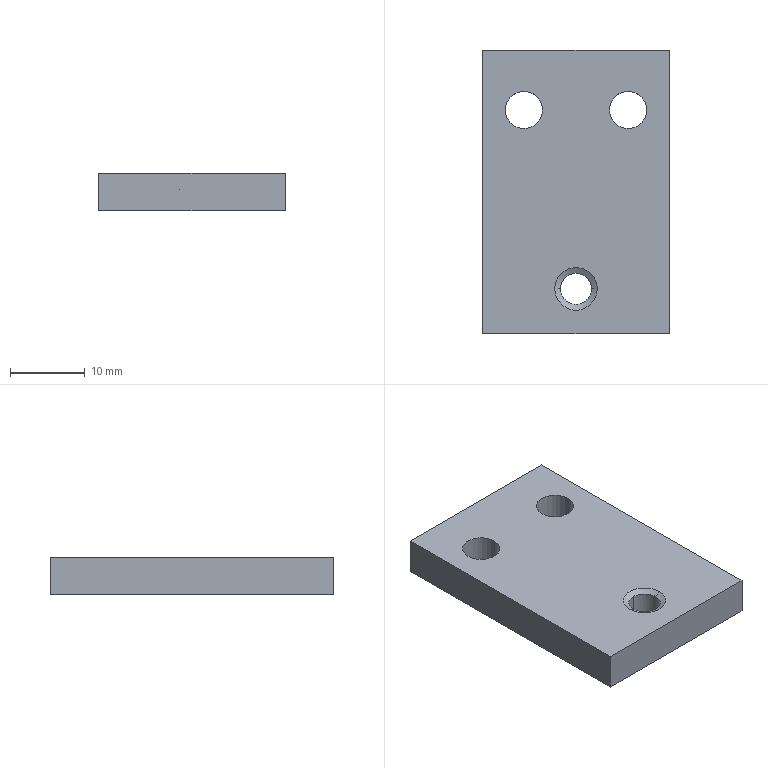Part | NX | 1 solid | 14 faces | box 25 x 38 x 5 mm | volume 4482 mm3 | plane 6 | cylinder 6 | cone 2 | commonest cylinder face diameters 5 x4 4.2 x2
STEP:
#1=CARTESIAN_POINT('',(-12.5,-20.5,-2.5));
#2=VERTEX_POINT('',#1);
#3=CARTESIAN_POINT('',(-12.5,17.5,-2.5));
#4=VERTEX_POINT('',#3);
#5=CARTESIAN_POINT('',(-12.5,0.,-2.5));
#6=DIRECTION('',(0.,1.,0.));
#7=VECTOR('',#6,1000.);
#8=LINE('',#5,#7);
#9=EDGE_CURVE('',#2,#4,#8,.T.);
#10=ORIENTED_EDGE('',*,*,#9,.T.);
#11=CARTESIAN_POINT('',(12.5,17.5,-2.5));
#12=VERTEX_POINT('',#11);
#13=CARTESIAN_POINT('',(0.,17.5,-2.5));
#14=DIRECTION('',(-1.,0.,0.));
#15=VECTOR('',#14,1000.);
#16=LINE('',#13,#15);
#17=EDGE_CURVE('',#12,#4,#16,.T.);
#18=ORIENTED_EDGE('',*,*,#17,.F.);
#19=CARTESIAN_POINT('',(12.5,-20.5,-2.5));
#20=VERTEX_POINT('',#19);
#21=CARTESIAN_POINT('',(12.5,0.,-2.5));
#22=DIRECTION('',(0.,-1.,0.));
#23=VECTOR('',#22,1000.);
#24=LINE('',#21,#23);
#25=EDGE_CURVE('',#12,#20,#24,.T.);
#26=ORIENTED_EDGE('',*,*,#25,.T.);
#27=CARTESIAN_POINT('',(0.,-20.5,-2.5));
#28=DIRECTION('',(1.,0.,0.));
#29=VECTOR('',#28,1000.);
#30=LINE('',#27,#29);
#31=EDGE_CURVE('',#2,#20,#30,.T.);
#32=ORIENTED_EDGE('',*,*,#31,.F.);
#33=EDGE_LOOP('',(#10,#18,#26,#32));
#34=FACE_BOUND('',#33,.T.);
#35=CARTESIAN_POINT('',(-4.5,9.5,-2.5));
#36=VERTEX_POINT('',#35);
#37=CARTESIAN_POINT('',(-9.5,9.5,-2.5));
#38=VERTEX_POINT('',#37);
#39=CARTESIAN_POINT('',(-7.,9.5,-2.5));
#40=DIRECTION('',(0.,0.,-1.));
#41=DIRECTION('',(-1.,0.,0.));
#42=AXIS2_PLACEMENT_3D('',#39,#40,#41);
#43=CIRCLE('',#42,2.5);
#44=EDGE_CURVE('',#36,#38,#43,.T.);
#45=ORIENTED_EDGE('',*,*,#44,.F.);
#46=CARTESIAN_POINT('',(-7.,9.5,-2.5));
#47=DIRECTION('',(0.,0.,-1.));
#48=DIRECTION('',(-1.,0.,0.));
#49=AXIS2_PLACEMENT_3D('',#46,#47,#48);
#50=CIRCLE('',#49,2.5);
#51=EDGE_CURVE('',#38,#36,#50,.T.);
#52=ORIENTED_EDGE('',*,*,#51,.F.);
#53=EDGE_LOOP('',(#45,#52));
#54=FACE_BOUND('',#53,.T.);
#55=CARTESIAN_POINT('',(0.,-12.4,-2.5));
#56=VERTEX_POINT('',#55);
#57=CARTESIAN_POINT('',(0.,-16.6,-2.5));
#58=VERTEX_POINT('',#57);
#59=CARTESIAN_POINT('',(0.,-14.5,-2.5));
#60=DIRECTION('',(0.,0.,1.));
#61=DIRECTION('',(0.,-1.,0.));
#62=AXIS2_PLACEMENT_3D('',#59,#60,#61);
#63=CIRCLE('',#62,2.1);
#64=EDGE_CURVE('',#56,#58,#63,.T.);
#65=ORIENTED_EDGE('',*,*,#64,.T.);
#66=CARTESIAN_POINT('',(0.,-14.5,-2.5));
#67=DIRECTION('',(0.,0.,1.));
#68=DIRECTION('',(0.,-1.,0.));
#69=AXIS2_PLACEMENT_3D('',#66,#67,#68);
#70=CIRCLE('',#69,2.1);
#71=EDGE_CURVE('',#58,#56,#70,.T.);
#72=ORIENTED_EDGE('',*,*,#71,.T.);
#73=EDGE_LOOP('',(#65,#72));
#74=FACE_BOUND('',#73,.T.);
#75=CARTESIAN_POINT('',(4.5,9.5,-2.5));
#76=VERTEX_POINT('',#75);
#77=CARTESIAN_POINT('',(9.5,9.5,-2.5));
#78=VERTEX_POINT('',#77);
#79=CARTESIAN_POINT('',(7.,9.5,-2.5));
#80=DIRECTION('',(0.,0.,-1.));
#81=DIRECTION('',(-1.,0.,0.));
#82=AXIS2_PLACEMENT_3D('',#79,#80,#81);
#83=CIRCLE('',#82,2.5);
#84=EDGE_CURVE('',#76,#78,#83,.T.);
#85=ORIENTED_EDGE('',*,*,#84,.F.);
#86=CARTESIAN_POINT('',(7.,9.5,-2.5));
#87=DIRECTION('',(0.,0.,-1.));
#88=DIRECTION('',(-1.,0.,0.));
#89=AXIS2_PLACEMENT_3D('',#86,#87,#88);
#90=CIRCLE('',#89,2.5);
#91=EDGE_CURVE('',#78,#76,#90,.T.);
#92=ORIENTED_EDGE('',*,*,#91,.F.);
#93=EDGE_LOOP('',(#85,#92));
#94=FACE_BOUND('',#93,.T.);
#95=CARTESIAN_POINT('',(0.,0.,-2.5));
#96=DIRECTION('',(0.,0.,1.));
#97=DIRECTION('',(1.,0.,0.));
#98=AXIS2_PLACEMENT_3D('',#95,#96,#97);
#99=PLANE('',#98);
#100=ADVANCED_FACE('',(#34,#54,#74,#94),#99,.F.);
#101=ORIENTED_EDGE('',*,*,#9,.F.);
#102=CARTESIAN_POINT('',(-12.5,-20.5,2.5));
#103=VERTEX_POINT('',#102);
#104=CARTESIAN_POINT('',(-12.5,-20.5,0.));
#105=DIRECTION('',(0.,0.,1.));
#106=VECTOR('',#105,1000.);
#107=LINE('',#104,#106);
#108=EDGE_CURVE('',#2,#103,#107,.T.);
#109=ORIENTED_EDGE('',*,*,#108,.T.);
#110=CARTESIAN_POINT('',(-12.5,17.5,2.5));
#111=VERTEX_POINT('',#110);
#112=CARTESIAN_POINT('',(-12.5,0.,2.5));
#113=DIRECTION('',(0.,1.,0.));
#114=VECTOR('',#113,1000.);
#115=LINE('',#112,#114);
#116=EDGE_CURVE('',#103,#111,#115,.T.);
#117=ORIENTED_EDGE('',*,*,#116,.T.);
#118=CARTESIAN_POINT('',(-12.5,17.5,0.));
#119=DIRECTION('',(0.,0.,-1.));
#120=VECTOR('',#119,1000.);
#121=LINE('',#118,#120);
#122=EDGE_CURVE('',#111,#4,#121,.T.);
#123=ORIENTED_EDGE('',*,*,#122,.T.);
#124=EDGE_LOOP('',(#101,#109,#117,#123));
#125=FACE_BOUND('',#124,.T.);
#126=CARTESIAN_POINT('',(-12.5,18.,-2.5));
#127=DIRECTION('',(-1.,0.,0.));
#128=DIRECTION('',(0.,0.,1.));
#129=AXIS2_PLACEMENT_3D('',#126,#127,#128);
#130=PLANE('',#129);
#131=ADVANCED_FACE('',(#125),#130,.T.);
#132=ORIENTED_EDGE('',*,*,#17,.T.);
#133=ORIENTED_EDGE('',*,*,#122,.F.);
#134=CARTESIAN_POINT('',(12.5,17.5,2.5));
#135=VERTEX_POINT('',#134);
#136=CARTESIAN_POINT('',(0.,17.5,2.5));
#137=DIRECTION('',(-1.,0.,0.));
#138=VECTOR('',#137,1000.);
#139=LINE('',#136,#138);
#140=EDGE_CURVE('',#135,#111,#139,.T.);
#141=ORIENTED_EDGE('',*,*,#140,.F.);
#142=CARTESIAN_POINT('',(12.5,17.5,0.));
#143=DIRECTION('',(0.,0.,1.));
#144=VECTOR('',#143,1000.);
#145=LINE('',#142,#144);
#146=EDGE_CURVE('',#12,#135,#145,.T.);
#147=ORIENTED_EDGE('',*,*,#146,.F.);
#148=EDGE_LOOP('',(#132,#133,#141,#147));
#149=FACE_BOUND('',#148,.T.);
#150=CARTESIAN_POINT('',(205.,17.5,-99.5));
#151=DIRECTION('',(0.,-1.,0.));
#152=DIRECTION('',(0.,0.,-1.));
#153=AXIS2_PLACEMENT_3D('',#150,#151,#152);
#154=PLANE('',#153);
#155=ADVANCED_FACE('',(#149),#154,.F.);
#156=ORIENTED_EDGE('',*,*,#25,.F.);
#157=ORIENTED_EDGE('',*,*,#146,.T.);
#158=CARTESIAN_POINT('',(12.5,-20.5,2.5));
#159=VERTEX_POINT('',#158);
#160=CARTESIAN_POINT('',(12.5,0.,2.5));
#161=DIRECTION('',(0.,-1.,0.));
#162=VECTOR('',#161,1000.);
#163=LINE('',#160,#162);
#164=EDGE_CURVE('',#135,#159,#163,.T.);
#165=ORIENTED_EDGE('',*,*,#164,.T.);
#166=CARTESIAN_POINT('',(12.5,-20.5,0.));
#167=DIRECTION('',(0.,0.,-1.));
#168=VECTOR('',#167,1000.);
#169=LINE('',#166,#168);
#170=EDGE_CURVE('',#159,#20,#169,.T.);
#171=ORIENTED_EDGE('',*,*,#170,.T.);
#172=EDGE_LOOP('',(#156,#157,#165,#171));
#173=FACE_BOUND('',#172,.T.);
#174=CARTESIAN_POINT('',(12.5,-18.,-2.5));
#175=DIRECTION('',(1.,0.,0.));
#176=DIRECTION('',(0.,1.,0.));
#177=AXIS2_PLACEMENT_3D('',#174,#175,#176);
#178=PLANE('',#177);
#179=ADVANCED_FACE('',(#173),#178,.T.);
#180=ORIENTED_EDGE('',*,*,#31,.T.);
#181=ORIENTED_EDGE('',*,*,#170,.F.);
#182=CARTESIAN_POINT('',(0.,-20.5,2.5));
#183=DIRECTION('',(1.,0.,0.));
#184=VECTOR('',#183,1000.);
#185=LINE('',#182,#184);
#186=EDGE_CURVE('',#103,#159,#185,.T.);
#187=ORIENTED_EDGE('',*,*,#186,.F.);
#188=ORIENTED_EDGE('',*,*,#108,.F.);
#189=EDGE_LOOP('',(#180,#181,#187,#188));
#190=FACE_BOUND('',#189,.T.);
#191=CARTESIAN_POINT('',(-12.5,-20.5,-2.5));
#192=DIRECTION('',(0.,-1.,0.));
#193=DIRECTION('',(0.,0.,-1.));
#194=AXIS2_PLACEMENT_3D('',#191,#192,#193);
#195=PLANE('',#194);
#196=ADVANCED_FACE('',(#190),#195,.T.);
#197=ORIENTED_EDGE('',*,*,#116,.F.);
#198=ORIENTED_EDGE('',*,*,#186,.T.);
#199=ORIENTED_EDGE('',*,*,#164,.F.);
#200=ORIENTED_EDGE('',*,*,#140,.T.);
#201=EDGE_LOOP('',(#197,#198,#199,#200));
#202=FACE_BOUND('',#201,.T.);
#203=CARTESIAN_POINT('',(-9.5,9.5,2.5));
#204=VERTEX_POINT('',#203);
#205=CARTESIAN_POINT('',(-4.5,9.5,2.5));
#206=VERTEX_POINT('',#205);
#207=CARTESIAN_POINT('',(-7.,9.5,2.5));
#208=DIRECTION('',(0.,0.,-1.));
#209=DIRECTION('',(-1.,0.,0.));
#210=AXIS2_PLACEMENT_3D('',#207,#208,#209);
#211=CIRCLE('',#210,2.5);
#212=EDGE_CURVE('',#204,#206,#211,.T.);
#213=ORIENTED_EDGE('',*,*,#212,.T.);
#214=CARTESIAN_POINT('',(-7.,9.5,2.5));
#215=DIRECTION('',(0.,0.,-1.));
#216=DIRECTION('',(-1.,0.,0.));
#217=AXIS2_PLACEMENT_3D('',#214,#215,#216);
#218=CIRCLE('',#217,2.5);
#219=EDGE_CURVE('',#206,#204,#218,.T.);
#220=ORIENTED_EDGE('',*,*,#219,.T.);
#221=EDGE_LOOP('',(#213,#220));
#222=FACE_BOUND('',#221,.T.);
#223=CARTESIAN_POINT('',(9.5,9.5,2.5));
#224=VERTEX_POINT('',#223);
#225=CARTESIAN_POINT('',(4.5,9.5,2.5));
#226=VERTEX_POINT('',#225);
#227=CARTESIAN_POINT('',(7.,9.5,2.5));
#228=DIRECTION('',(0.,0.,-1.));
#229=DIRECTION('',(-1.,0.,0.));
#230=AXIS2_PLACEMENT_3D('',#227,#228,#229);
#231=CIRCLE('',#230,2.5);
#232=EDGE_CURVE('',#224,#226,#231,.T.);
#233=ORIENTED_EDGE('',*,*,#232,.T.);
#234=CARTESIAN_POINT('',(7.,9.5,2.5));
#235=DIRECTION('',(0.,0.,-1.));
#236=DIRECTION('',(-1.,0.,0.));
#237=AXIS2_PLACEMENT_3D('',#234,#235,#236);
#238=CIRCLE('',#237,2.5);
#239=EDGE_CURVE('',#226,#224,#238,.T.);
#240=ORIENTED_EDGE('',*,*,#239,.T.);
#241=EDGE_LOOP('',(#233,#240));
#242=FACE_BOUND('',#241,.T.);
#243=CARTESIAN_POINT('',(2.86,-14.5,2.5));
#244=VERTEX_POINT('',#243);
#245=CARTESIAN_POINT('',(-2.86,-14.5,2.5));
#246=VERTEX_POINT('',#245);
#247=CARTESIAN_POINT('',(0.,-14.5,2.5));
#248=DIRECTION('',(0.,0.,1.));
#249=DIRECTION('',(1.,0.,0.));
#250=AXIS2_PLACEMENT_3D('',#247,#248,#249);
#251=CIRCLE('',#250,2.86);
#252=EDGE_CURVE('',#244,#246,#251,.T.);
#253=ORIENTED_EDGE('',*,*,#252,.F.);
#254=CARTESIAN_POINT('',(0.,-14.5,2.5));
#255=DIRECTION('',(0.,0.,1.));
#256=DIRECTION('',(1.,0.,0.));
#257=AXIS2_PLACEMENT_3D('',#254,#255,#256);
#258=CIRCLE('',#257,2.86);
#259=EDGE_CURVE('',#246,#244,#258,.T.);
#260=ORIENTED_EDGE('',*,*,#259,.F.);
#261=EDGE_LOOP('',(#253,#260));
#262=FACE_BOUND('',#261,.T.);
#263=CARTESIAN_POINT('',(0.,0.,2.5));
#264=DIRECTION('',(0.,0.,1.));
#265=DIRECTION('',(1.,0.,0.));
#266=AXIS2_PLACEMENT_3D('',#263,#264,#265);
#267=PLANE('',#266);
#268=ADVANCED_FACE('',(#202,#222,#242,#262),#267,.T.);
#269=ORIENTED_EDGE('',*,*,#212,.F.);
#270=CARTESIAN_POINT('',(-9.5,9.5,2.5));
#271=DIRECTION('',(0.,0.,-1.));
#272=VECTOR('',#271,1000.);
#273=LINE('',#270,#272);
#274=EDGE_CURVE('',#38,#204,#273,.F.);
#275=ORIENTED_EDGE('',*,*,#274,.F.);
#276=ORIENTED_EDGE('',*,*,#51,.T.);
#277=CARTESIAN_POINT('',(-4.5,9.5,2.5));
#278=DIRECTION('',(0.,0.,-1.));
#279=VECTOR('',#278,1000.);
#280=LINE('',#277,#279);
#281=EDGE_CURVE('',#36,#206,#280,.F.);
#282=ORIENTED_EDGE('',*,*,#281,.T.);
#283=EDGE_LOOP('',(#269,#275,#276,#282));
#284=FACE_BOUND('',#283,.T.);
#285=CARTESIAN_POINT('',(-7.,9.5,2.5));
#286=DIRECTION('',(0.,0.,-1.));
#287=DIRECTION('',(-1.,0.,0.));
#288=AXIS2_PLACEMENT_3D('',#285,#286,#287);
#289=CYLINDRICAL_SURFACE('',#288,2.5);
#290=ADVANCED_FACE('',(#284),#289,.F.);
#291=ORIENTED_EDGE('',*,*,#232,.F.);
#292=CARTESIAN_POINT('',(9.5,9.5,2.5));
#293=DIRECTION('',(0.,0.,-1.));
#294=VECTOR('',#293,1000.);
#295=LINE('',#292,#294);
#296=EDGE_CURVE('',#224,#78,#295,.T.);
#297=ORIENTED_EDGE('',*,*,#296,.T.);
#298=ORIENTED_EDGE('',*,*,#91,.T.);
#299=CARTESIAN_POINT('',(4.5,9.5,2.5));
#300=DIRECTION('',(0.,0.,-1.));
#301=VECTOR('',#300,1000.);
#302=LINE('',#299,#301);
#303=EDGE_CURVE('',#226,#76,#302,.T.);
#304=ORIENTED_EDGE('',*,*,#303,.F.);
#305=EDGE_LOOP('',(#291,#297,#298,#304));
#306=FACE_BOUND('',#305,.T.);
#307=CARTESIAN_POINT('',(7.,9.5,2.5));
#308=DIRECTION('',(0.,0.,-1.));
#309=DIRECTION('',(-1.,0.,0.));
#310=AXIS2_PLACEMENT_3D('',#307,#308,#309);
#311=CYLINDRICAL_SURFACE('',#310,2.5);
#312=ADVANCED_FACE('',(#306),#311,.F.);
#313=CARTESIAN_POINT('',(0.,-12.4,2.061));
#314=VERTEX_POINT('',#313);
#315=CARTESIAN_POINT('',(-2.1,-14.5,2.061));
#316=VERTEX_POINT('',#315);
#317=CARTESIAN_POINT('',(0.,-14.5,2.061));
#318=DIRECTION('',(0.,0.,1.));
#319=DIRECTION('',(1.,0.,0.));
#320=AXIS2_PLACEMENT_3D('',#317,#318,#319);
#321=CIRCLE('',#320,2.1);
#322=EDGE_CURVE('',#314,#316,#321,.T.);
#323=ORIENTED_EDGE('',*,*,#322,.T.);
#324=CARTESIAN_POINT('',(0.,-16.6,2.061));
#325=VERTEX_POINT('',#324);
#326=CARTESIAN_POINT('',(0.,-14.5,2.061));
#327=DIRECTION('',(0.,0.,1.));
#328=DIRECTION('',(1.,0.,0.));
#329=AXIS2_PLACEMENT_3D('',#326,#327,#328);
#330=CIRCLE('',#329,2.1);
#331=EDGE_CURVE('',#316,#325,#330,.T.);
#332=ORIENTED_EDGE('',*,*,#331,.T.);
#333=CARTESIAN_POINT('',(0.,-16.6,0.));
#334=DIRECTION('',(0.,0.,1.));
#335=VECTOR('',#334,1000.);
#336=LINE('',#333,#335);
#337=EDGE_CURVE('',#325,#58,#336,.F.);
#338=ORIENTED_EDGE('',*,*,#337,.T.);
#339=ORIENTED_EDGE('',*,*,#64,.F.);
#340=CARTESIAN_POINT('',(0.,-12.4,0.));
#341=DIRECTION('',(0.,0.,1.));
#342=VECTOR('',#341,1000.);
#343=LINE('',#340,#342);
#344=EDGE_CURVE('',#314,#56,#343,.F.);
#345=ORIENTED_EDGE('',*,*,#344,.F.);
#346=EDGE_LOOP('',(#323,#332,#338,#339,#345));
#347=FACE_BOUND('',#346,.T.);
#348=CARTESIAN_POINT('',(0.,-14.5,0.));
#349=DIRECTION('',(0.,0.,1.));
#350=DIRECTION('',(0.,-1.,0.));
#351=AXIS2_PLACEMENT_3D('',#348,#349,#350);
#352=CYLINDRICAL_SURFACE('',#351,2.1);
#353=ADVANCED_FACE('',(#347),#352,.F.);
#354=ORIENTED_EDGE('',*,*,#252,.T.);
#355=CARTESIAN_POINT('',(-2.1,-14.5,2.061));
#356=DIRECTION('',(-0.866,0.,0.5));
#357=VECTOR('',#356,1000.);
#358=LINE('',#355,#357);
#359=EDGE_CURVE('',#316,#246,#358,.T.);
#360=ORIENTED_EDGE('',*,*,#359,.F.);
#361=ORIENTED_EDGE('',*,*,#322,.F.);
#362=CARTESIAN_POINT('',(2.1,-14.5,2.061));
#363=VERTEX_POINT('',#362);
#364=CARTESIAN_POINT('',(0.,-14.5,2.061));
#365=DIRECTION('',(0.,0.,1.));
#366=DIRECTION('',(1.,0.,0.));
#367=AXIS2_PLACEMENT_3D('',#364,#365,#366);
#368=CIRCLE('',#367,2.1);
#369=EDGE_CURVE('',#363,#314,#368,.T.);
#370=ORIENTED_EDGE('',*,*,#369,.F.);
#371=CARTESIAN_POINT('',(2.1,-14.5,2.061));
#372=DIRECTION('',(0.866,0.,0.5));
#373=VECTOR('',#372,1000.);
#374=LINE('',#371,#373);
#375=EDGE_CURVE('',#363,#244,#374,.T.);
#376=ORIENTED_EDGE('',*,*,#375,.T.);
#377=EDGE_LOOP('',(#354,#360,#361,#370,#376));
#378=FACE_BOUND('',#377,.T.);
#379=CARTESIAN_POINT('',(0.,-14.5,2.061));
#380=DIRECTION('',(0.,0.,1.));
#381=DIRECTION('',(1.,0.,0.));
#382=AXIS2_PLACEMENT_3D('',#379,#380,#381);
#383=CONICAL_SURFACE('',#382,2.1,1.047);
#384=ADVANCED_FACE('',(#378),#383,.F.);
#385=ORIENTED_EDGE('',*,*,#337,.F.);
#386=CARTESIAN_POINT('',(0.,-14.5,2.061));
#387=DIRECTION('',(0.,0.,1.));
#388=DIRECTION('',(1.,0.,0.));
#389=AXIS2_PLACEMENT_3D('',#386,#387,#388);
#390=CIRCLE('',#389,2.1);
#391=EDGE_CURVE('',#325,#363,#390,.T.);
#392=ORIENTED_EDGE('',*,*,#391,.T.);
#393=ORIENTED_EDGE('',*,*,#369,.T.);
#394=ORIENTED_EDGE('',*,*,#344,.T.);
#395=ORIENTED_EDGE('',*,*,#71,.F.);
#396=EDGE_LOOP('',(#385,#392,#393,#394,#395));
#397=FACE_BOUND('',#396,.T.);
#398=CARTESIAN_POINT('',(0.,-14.5,0.));
#399=DIRECTION('',(0.,0.,1.));
#400=DIRECTION('',(0.,-1.,0.));
#401=AXIS2_PLACEMENT_3D('',#398,#399,#400);
#402=CYLINDRICAL_SURFACE('',#401,2.1);
#403=ADVANCED_FACE('',(#397),#402,.F.);
#404=ORIENTED_EDGE('',*,*,#375,.F.);
#405=ORIENTED_EDGE('',*,*,#391,.F.);
#406=ORIENTED_EDGE('',*,*,#331,.F.);
#407=ORIENTED_EDGE('',*,*,#359,.T.);
#408=ORIENTED_EDGE('',*,*,#259,.T.);
#409=EDGE_LOOP('',(#404,#405,#406,#407,#408));
#410=FACE_BOUND('',#409,.T.);
#411=CARTESIAN_POINT('',(0.,-14.5,2.061));
#412=DIRECTION('',(0.,0.,1.));
#413=DIRECTION('',(1.,0.,0.));
#414=AXIS2_PLACEMENT_3D('',#411,#412,#413);
#415=CONICAL_SURFACE('',#414,2.1,1.047);
#416=ADVANCED_FACE('',(#410),#415,.F.);
#417=ORIENTED_EDGE('',*,*,#84,.T.);
#418=ORIENTED_EDGE('',*,*,#296,.F.);
#419=ORIENTED_EDGE('',*,*,#239,.F.);
#420=ORIENTED_EDGE('',*,*,#303,.T.);
#421=EDGE_LOOP('',(#417,#418,#419,#420));
#422=FACE_BOUND('',#421,.T.);
#423=CARTESIAN_POINT('',(7.,9.5,2.5));
#424=DIRECTION('',(0.,0.,-1.));
#425=DIRECTION('',(-1.,0.,0.));
#426=AXIS2_PLACEMENT_3D('',#423,#424,#425);
#427=CYLINDRICAL_SURFACE('',#426,2.5);
#428=ADVANCED_FACE('',(#422),#427,.F.);
#429=ORIENTED_EDGE('',*,*,#44,.T.);
#430=ORIENTED_EDGE('',*,*,#274,.T.);
#431=ORIENTED_EDGE('',*,*,#219,.F.);
#432=ORIENTED_EDGE('',*,*,#281,.F.);
#433=EDGE_LOOP('',(#429,#430,#431,#432));
#434=FACE_BOUND('',#433,.T.);
#435=CARTESIAN_POINT('',(-7.,9.5,2.5));
#436=DIRECTION('',(0.,0.,-1.));
#437=DIRECTION('',(-1.,0.,0.));
#438=AXIS2_PLACEMENT_3D('',#435,#436,#437);
#439=CYLINDRICAL_SURFACE('',#438,2.5);
#440=ADVANCED_FACE('',(#434),#439,.F.);
#441=CLOSED_SHELL('',(#100,#131,#155,#179,#196,#268,#290,#312,#353,#384,#403,#416,#428,#440));
#442=MANIFOLD_SOLID_BREP('',#441);
#443=(LENGTH_UNIT()NAMED_UNIT(*)SI_UNIT(.MILLI.,.METRE.));
#444=UNCERTAINTY_MEASURE_WITH_UNIT(LENGTH_MEASURE(0.00001),#443,'','');
#445=(NAMED_UNIT(*)PLANE_ANGLE_UNIT()SI_UNIT($,.RADIAN.));
#446=(NAMED_UNIT(*)SI_UNIT($,.STERADIAN.)SOLID_ANGLE_UNIT());
#447=(GEOMETRIC_REPRESENTATION_CONTEXT(3)GLOBAL_UNCERTAINTY_ASSIGNED_CONTEXT((#444))GLOBAL_UNIT_ASSIGNED_CONTEXT((#443,#445,#446))REPRESENTATION_CONTEXT('',''));
#448=ADVANCED_BREP_SHAPE_REPRESENTATION('',(#442),#447);